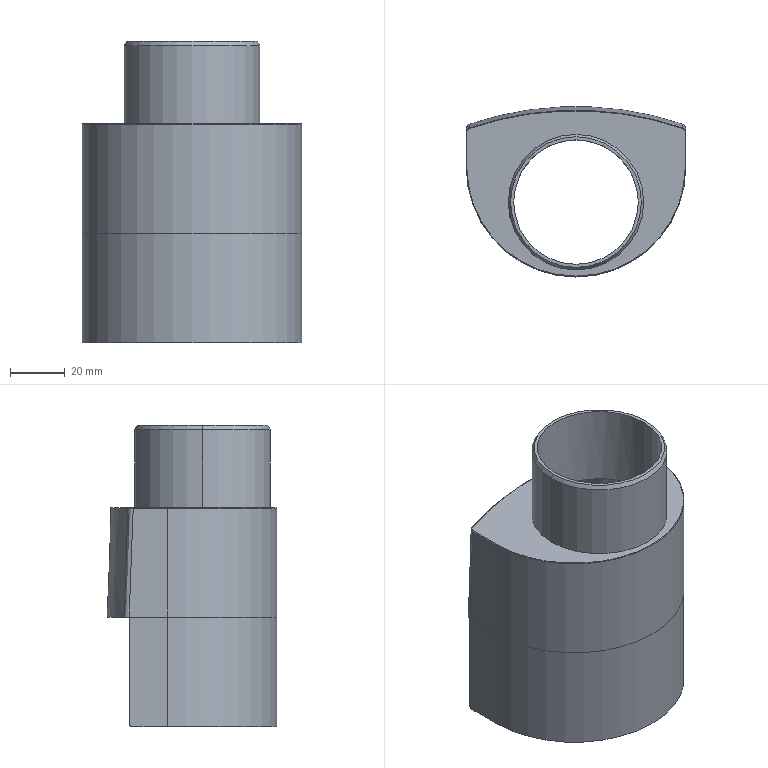Part | STEP file | Ice maker outlet adapter 001 | 2 solids | 36 faces | box 80.19 x 62.19 x 110 mm | volume 80643 mm3 | plane 13 | cylinder 11 | spline 7 | cone 3 | torus 2 | commonest cylinder face diameters 0.4 x2 2 x2 45.5 x2 49.5 x2 80.19 x2 76.19 x1